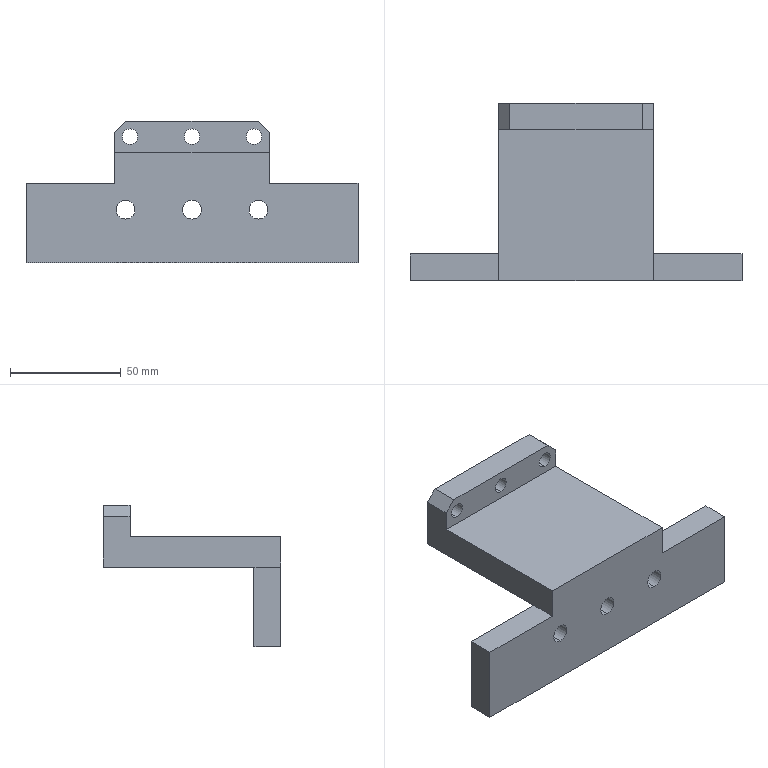Part | NX | 1 solid | 28 faces | box 150 x 80 x 64 mm | volume 151232 mm3 | plane 16 | cylinder 12 | commonest cylinder face diameters 7 x6 8.5 x6
STEP:
#1=CARTESIAN_POINT('',(0.,-28.,-35.75));
#2=VERTEX_POINT('',#1);
#3=CARTESIAN_POINT('',(0.,-28.,-44.25));
#4=VERTEX_POINT('',#3);
#5=CARTESIAN_POINT('',(0.,-28.,-40.));
#6=DIRECTION('',(0.,-1.,0.));
#7=DIRECTION('',(0.,0.,-1.));
#8=AXIS2_PLACEMENT_3D('',#5,#6,#7);
#9=CIRCLE('',#8,4.25);
#10=EDGE_CURVE('',#2,#4,#9,.T.);
#11=ORIENTED_EDGE('',*,*,#10,.F.);
#12=CARTESIAN_POINT('',(0.,-40.,-35.75));
#13=VERTEX_POINT('',#12);
#14=CARTESIAN_POINT('',(0.,-40.,-35.75));
#15=DIRECTION('',(0.,-1.,0.));
#16=VECTOR('',#15,1000.);
#17=LINE('',#14,#16);
#18=EDGE_CURVE('',#2,#13,#17,.T.);
#19=ORIENTED_EDGE('',*,*,#18,.T.);
#20=CARTESIAN_POINT('',(0.,-40.,-44.25));
#21=VERTEX_POINT('',#20);
#22=CARTESIAN_POINT('',(0.,-40.,-40.));
#23=DIRECTION('',(0.,-1.,0.));
#24=DIRECTION('',(0.,0.,-1.));
#25=AXIS2_PLACEMENT_3D('',#22,#23,#24);
#26=CIRCLE('',#25,4.25);
#27=EDGE_CURVE('',#13,#21,#26,.T.);
#28=ORIENTED_EDGE('',*,*,#27,.T.);
#29=CARTESIAN_POINT('',(0.,-40.,-44.25));
#30=DIRECTION('',(0.,-1.,0.));
#31=VECTOR('',#30,1000.);
#32=LINE('',#29,#31);
#33=EDGE_CURVE('',#4,#21,#32,.T.);
#34=ORIENTED_EDGE('',*,*,#33,.F.);
#35=EDGE_LOOP('',(#11,#19,#28,#34));
#36=FACE_BOUND('',#35,.T.);
#37=CARTESIAN_POINT('',(0.,-40.,-40.));
#38=DIRECTION('',(0.,-1.,0.));
#39=DIRECTION('',(0.,0.,1.));
#40=AXIS2_PLACEMENT_3D('',#37,#38,#39);
#41=CYLINDRICAL_SURFACE('',#40,4.25);
#42=ADVANCED_FACE('',(#36),#41,.F.);
#43=CARTESIAN_POINT('',(30.,-28.,-35.75));
#44=VERTEX_POINT('',#43);
#45=CARTESIAN_POINT('',(30.,-28.,-44.25));
#46=VERTEX_POINT('',#45);
#47=CARTESIAN_POINT('',(30.,-28.,-40.));
#48=DIRECTION('',(0.,-1.,0.));
#49=DIRECTION('',(0.,0.,-1.));
#50=AXIS2_PLACEMENT_3D('',#47,#48,#49);
#51=CIRCLE('',#50,4.25);
#52=EDGE_CURVE('',#44,#46,#51,.T.);
#53=ORIENTED_EDGE('',*,*,#52,.F.);
#54=CARTESIAN_POINT('',(30.,-40.,-35.75));
#55=VERTEX_POINT('',#54);
#56=CARTESIAN_POINT('',(30.,-40.,-35.75));
#57=DIRECTION('',(0.,-1.,0.));
#58=VECTOR('',#57,1000.);
#59=LINE('',#56,#58);
#60=EDGE_CURVE('',#44,#55,#59,.T.);
#61=ORIENTED_EDGE('',*,*,#60,.T.);
#62=CARTESIAN_POINT('',(30.,-40.,-44.25));
#63=VERTEX_POINT('',#62);
#64=CARTESIAN_POINT('',(30.,-40.,-40.));
#65=DIRECTION('',(0.,-1.,0.));
#66=DIRECTION('',(0.,0.,-1.));
#67=AXIS2_PLACEMENT_3D('',#64,#65,#66);
#68=CIRCLE('',#67,4.25);
#69=EDGE_CURVE('',#55,#63,#68,.T.);
#70=ORIENTED_EDGE('',*,*,#69,.T.);
#71=CARTESIAN_POINT('',(30.,-40.,-44.25));
#72=DIRECTION('',(0.,-1.,0.));
#73=VECTOR('',#72,1000.);
#74=LINE('',#71,#73);
#75=EDGE_CURVE('',#46,#63,#74,.T.);
#76=ORIENTED_EDGE('',*,*,#75,.F.);
#77=EDGE_LOOP('',(#53,#61,#70,#76));
#78=FACE_BOUND('',#77,.T.);
#79=CARTESIAN_POINT('',(30.,-40.,-40.));
#80=DIRECTION('',(0.,-1.,0.));
#81=DIRECTION('',(0.,0.,1.));
#82=AXIS2_PLACEMENT_3D('',#79,#80,#81);
#83=CYLINDRICAL_SURFACE('',#82,4.25);
#84=ADVANCED_FACE('',(#78),#83,.F.);
#85=CARTESIAN_POINT('',(-28.,28.,-10.5));
#86=VERTEX_POINT('',#85);
#87=CARTESIAN_POINT('',(-28.,28.,-3.5));
#88=VERTEX_POINT('',#87);
#89=CARTESIAN_POINT('',(-28.,28.,-7.));
#90=DIRECTION('',(0.,1.,0.));
#91=DIRECTION('',(0.,0.,1.));
#92=AXIS2_PLACEMENT_3D('',#89,#90,#91);
#93=CIRCLE('',#92,3.5);
#94=EDGE_CURVE('',#86,#88,#93,.T.);
#95=ORIENTED_EDGE('',*,*,#94,.F.);
#96=CARTESIAN_POINT('',(-28.,40.,-10.5));
#97=VERTEX_POINT('',#96);
#98=CARTESIAN_POINT('',(-28.,40.,-10.5));
#99=DIRECTION('',(0.,1.,0.));
#100=VECTOR('',#99,1000.);
#101=LINE('',#98,#100);
#102=EDGE_CURVE('',#86,#97,#101,.T.);
#103=ORIENTED_EDGE('',*,*,#102,.T.);
#104=CARTESIAN_POINT('',(-28.,40.,-3.5));
#105=VERTEX_POINT('',#104);
#106=CARTESIAN_POINT('',(-28.,40.,-7.));
#107=DIRECTION('',(0.,1.,0.));
#108=DIRECTION('',(0.,0.,1.));
#109=AXIS2_PLACEMENT_3D('',#106,#107,#108);
#110=CIRCLE('',#109,3.5);
#111=EDGE_CURVE('',#97,#105,#110,.T.);
#112=ORIENTED_EDGE('',*,*,#111,.T.);
#113=CARTESIAN_POINT('',(-28.,40.,-3.5));
#114=DIRECTION('',(0.,1.,0.));
#115=VECTOR('',#114,1000.);
#116=LINE('',#113,#115);
#117=EDGE_CURVE('',#88,#105,#116,.T.);
#118=ORIENTED_EDGE('',*,*,#117,.F.);
#119=EDGE_LOOP('',(#95,#103,#112,#118));
#120=FACE_BOUND('',#119,.T.);
#121=CARTESIAN_POINT('',(-28.,40.,-7.));
#122=DIRECTION('',(0.,1.,0.));
#123=DIRECTION('',(0.,0.,-1.));
#124=AXIS2_PLACEMENT_3D('',#121,#122,#123);
#125=CYLINDRICAL_SURFACE('',#124,3.5);
#126=ADVANCED_FACE('',(#120),#125,.F.);
#127=CARTESIAN_POINT('',(0.,28.,-10.5));
#128=VERTEX_POINT('',#127);
#129=CARTESIAN_POINT('',(0.,28.,-3.5));
#130=VERTEX_POINT('',#129);
#131=CARTESIAN_POINT('',(0.,28.,-7.));
#132=DIRECTION('',(0.,1.,0.));
#133=DIRECTION('',(0.,0.,1.));
#134=AXIS2_PLACEMENT_3D('',#131,#132,#133);
#135=CIRCLE('',#134,3.5);
#136=EDGE_CURVE('',#128,#130,#135,.T.);
#137=ORIENTED_EDGE('',*,*,#136,.F.);
#138=CARTESIAN_POINT('',(0.,40.,-10.5));
#139=VERTEX_POINT('',#138);
#140=CARTESIAN_POINT('',(0.,40.,-10.5));
#141=DIRECTION('',(0.,1.,0.));
#142=VECTOR('',#141,1000.);
#143=LINE('',#140,#142);
#144=EDGE_CURVE('',#128,#139,#143,.T.);
#145=ORIENTED_EDGE('',*,*,#144,.T.);
#146=CARTESIAN_POINT('',(0.,40.,-3.5));
#147=VERTEX_POINT('',#146);
#148=CARTESIAN_POINT('',(0.,40.,-7.));
#149=DIRECTION('',(0.,1.,0.));
#150=DIRECTION('',(0.,0.,1.));
#151=AXIS2_PLACEMENT_3D('',#148,#149,#150);
#152=CIRCLE('',#151,3.5);
#153=EDGE_CURVE('',#139,#147,#152,.T.);
#154=ORIENTED_EDGE('',*,*,#153,.T.);
#155=CARTESIAN_POINT('',(0.,40.,-3.5));
#156=DIRECTION('',(0.,1.,0.));
#157=VECTOR('',#156,1000.);
#158=LINE('',#155,#157);
#159=EDGE_CURVE('',#130,#147,#158,.T.);
#160=ORIENTED_EDGE('',*,*,#159,.F.);
#161=EDGE_LOOP('',(#137,#145,#154,#160));
#162=FACE_BOUND('',#161,.T.);
#163=CARTESIAN_POINT('',(0.,40.,-7.));
#164=DIRECTION('',(0.,1.,0.));
#165=DIRECTION('',(0.,0.,-1.));
#166=AXIS2_PLACEMENT_3D('',#163,#164,#165);
#167=CYLINDRICAL_SURFACE('',#166,3.5);
#168=ADVANCED_FACE('',(#162),#167,.F.);
#169=CARTESIAN_POINT('',(28.,28.,-10.5));
#170=VERTEX_POINT('',#169);
#171=CARTESIAN_POINT('',(28.,28.,-3.5));
#172=VERTEX_POINT('',#171);
#173=CARTESIAN_POINT('',(28.,28.,-7.));
#174=DIRECTION('',(0.,1.,0.));
#175=DIRECTION('',(0.,0.,1.));
#176=AXIS2_PLACEMENT_3D('',#173,#174,#175);
#177=CIRCLE('',#176,3.5);
#178=EDGE_CURVE('',#170,#172,#177,.T.);
#179=ORIENTED_EDGE('',*,*,#178,.F.);
#180=CARTESIAN_POINT('',(28.,40.,-10.5));
#181=VERTEX_POINT('',#180);
#182=CARTESIAN_POINT('',(28.,40.,-10.5));
#183=DIRECTION('',(0.,1.,0.));
#184=VECTOR('',#183,1000.);
#185=LINE('',#182,#184);
#186=EDGE_CURVE('',#170,#181,#185,.T.);
#187=ORIENTED_EDGE('',*,*,#186,.T.);
#188=CARTESIAN_POINT('',(28.,40.,-3.5));
#189=VERTEX_POINT('',#188);
#190=CARTESIAN_POINT('',(28.,40.,-7.));
#191=DIRECTION('',(0.,1.,0.));
#192=DIRECTION('',(0.,0.,1.));
#193=AXIS2_PLACEMENT_3D('',#190,#191,#192);
#194=CIRCLE('',#193,3.5);
#195=EDGE_CURVE('',#181,#189,#194,.T.);
#196=ORIENTED_EDGE('',*,*,#195,.T.);
#197=CARTESIAN_POINT('',(28.,40.,-3.5));
#198=DIRECTION('',(0.,1.,0.));
#199=VECTOR('',#198,1000.);
#200=LINE('',#197,#199);
#201=EDGE_CURVE('',#172,#189,#200,.T.);
#202=ORIENTED_EDGE('',*,*,#201,.F.);
#203=EDGE_LOOP('',(#179,#187,#196,#202));
#204=FACE_BOUND('',#203,.T.);
#205=CARTESIAN_POINT('',(28.,40.,-7.));
#206=DIRECTION('',(0.,1.,0.));
#207=DIRECTION('',(0.,0.,-1.));
#208=AXIS2_PLACEMENT_3D('',#205,#206,#207);
#209=CYLINDRICAL_SURFACE('',#208,3.5);
#210=ADVANCED_FACE('',(#204),#209,.F.);
#211=CARTESIAN_POINT('',(-30.,-28.,-35.75));
#212=VERTEX_POINT('',#211);
#213=CARTESIAN_POINT('',(-30.,-28.,-44.25));
#214=VERTEX_POINT('',#213);
#215=CARTESIAN_POINT('',(-30.,-28.,-40.));
#216=DIRECTION('',(0.,-1.,0.));
#217=DIRECTION('',(0.,0.,-1.));
#218=AXIS2_PLACEMENT_3D('',#215,#216,#217);
#219=CIRCLE('',#218,4.25);
#220=EDGE_CURVE('',#212,#214,#219,.T.);
#221=ORIENTED_EDGE('',*,*,#220,.F.);
#222=CARTESIAN_POINT('',(-30.,-40.,-35.75));
#223=VERTEX_POINT('',#222);
#224=CARTESIAN_POINT('',(-30.,-40.,-35.75));
#225=DIRECTION('',(0.,-1.,0.));
#226=VECTOR('',#225,1000.);
#227=LINE('',#224,#226);
#228=EDGE_CURVE('',#212,#223,#227,.T.);
#229=ORIENTED_EDGE('',*,*,#228,.T.);
#230=CARTESIAN_POINT('',(-30.,-40.,-44.25));
#231=VERTEX_POINT('',#230);
#232=CARTESIAN_POINT('',(-30.,-40.,-40.));
#233=DIRECTION('',(0.,-1.,0.));
#234=DIRECTION('',(0.,0.,-1.));
#235=AXIS2_PLACEMENT_3D('',#232,#233,#234);
#236=CIRCLE('',#235,4.25);
#237=EDGE_CURVE('',#223,#231,#236,.T.);
#238=ORIENTED_EDGE('',*,*,#237,.T.);
#239=CARTESIAN_POINT('',(-30.,-40.,-44.25));
#240=DIRECTION('',(0.,-1.,0.));
#241=VECTOR('',#240,1000.);
#242=LINE('',#239,#241);
#243=EDGE_CURVE('',#214,#231,#242,.T.);
#244=ORIENTED_EDGE('',*,*,#243,.F.);
#245=EDGE_LOOP('',(#221,#229,#238,#244));
#246=FACE_BOUND('',#245,.T.);
#247=CARTESIAN_POINT('',(-30.,-40.,-40.));
#248=DIRECTION('',(0.,-1.,0.));
#249=DIRECTION('',(0.,0.,1.));
#250=AXIS2_PLACEMENT_3D('',#247,#248,#249);
#251=CYLINDRICAL_SURFACE('',#250,4.25);
#252=ADVANCED_FACE('',(#246),#251,.F.);
#253=ORIENTED_EDGE('',*,*,#228,.F.);
#254=CARTESIAN_POINT('',(-30.,-28.,-40.));
#255=DIRECTION('',(0.,-1.,0.));
#256=DIRECTION('',(0.,0.,-1.));
#257=AXIS2_PLACEMENT_3D('',#254,#255,#256);
#258=CIRCLE('',#257,4.25);
#259=EDGE_CURVE('',#214,#212,#258,.T.);
#260=ORIENTED_EDGE('',*,*,#259,.F.);
#261=ORIENTED_EDGE('',*,*,#243,.T.);
#262=CARTESIAN_POINT('',(-30.,-40.,-40.));
#263=DIRECTION('',(0.,-1.,0.));
#264=DIRECTION('',(0.,0.,-1.));
#265=AXIS2_PLACEMENT_3D('',#262,#263,#264);
#266=CIRCLE('',#265,4.25);
#267=EDGE_CURVE('',#231,#223,#266,.T.);
#268=ORIENTED_EDGE('',*,*,#267,.T.);
#269=EDGE_LOOP('',(#253,#260,#261,#268));
#270=FACE_BOUND('',#269,.T.);
#271=CARTESIAN_POINT('',(-30.,-40.,-40.));
#272=DIRECTION('',(0.,-1.,0.));
#273=DIRECTION('',(0.,0.,1.));
#274=AXIS2_PLACEMENT_3D('',#271,#272,#273);
#275=CYLINDRICAL_SURFACE('',#274,4.25);
#276=ADVANCED_FACE('',(#270),#275,.F.);
#277=CARTESIAN_POINT('',(-75.,-40.,-64.));
#278=VERTEX_POINT('',#277);
#279=CARTESIAN_POINT('',(-75.,-40.,-28.));
#280=VERTEX_POINT('',#279);
#281=CARTESIAN_POINT('',(-75.,-40.,0.));
#282=DIRECTION('',(0.,0.,1.));
#283=VECTOR('',#282,1000.);
#284=LINE('',#281,#283);
#285=EDGE_CURVE('',#278,#280,#284,.T.);
#286=ORIENTED_EDGE('',*,*,#285,.T.);
#287=CARTESIAN_POINT('',(-75.,-28.,-28.));
#288=VERTEX_POINT('',#287);
#289=CARTESIAN_POINT('',(-75.,-40.,-28.));
#290=DIRECTION('',(0.,1.,0.));
#291=VECTOR('',#290,1000.);
#292=LINE('',#289,#291);
#293=EDGE_CURVE('',#280,#288,#292,.T.);
#294=ORIENTED_EDGE('',*,*,#293,.T.);
#295=CARTESIAN_POINT('',(-75.,-28.,-64.));
#296=VERTEX_POINT('',#295);
#297=CARTESIAN_POINT('',(-75.,-28.,-64.));
#298=DIRECTION('',(0.,0.,-1.));
#299=VECTOR('',#298,1000.);
#300=LINE('',#297,#299);
#301=EDGE_CURVE('',#288,#296,#300,.T.);
#302=ORIENTED_EDGE('',*,*,#301,.T.);
#303=CARTESIAN_POINT('',(-75.,40.,-64.));
#304=DIRECTION('',(0.,-1.,0.));
#305=VECTOR('',#304,1000.);
#306=LINE('',#303,#305);
#307=EDGE_CURVE('',#296,#278,#306,.T.);
#308=ORIENTED_EDGE('',*,*,#307,.T.);
#309=EDGE_LOOP('',(#286,#294,#302,#308));
#310=FACE_BOUND('',#309,.T.);
#311=CARTESIAN_POINT('',(-75.,40.,0.));
#312=DIRECTION('',(1.,0.,0.));
#313=DIRECTION('',(0.,0.,1.));
#314=AXIS2_PLACEMENT_3D('',#311,#312,#313);
#315=PLANE('',#314);
#316=ADVANCED_FACE('',(#310),#315,.F.);
#317=CARTESIAN_POINT('',(-30.,28.,0.));
#318=VERTEX_POINT('',#317);
#319=CARTESIAN_POINT('',(30.,28.,0.));
#320=VERTEX_POINT('',#319);
#321=CARTESIAN_POINT('',(-75.,28.,0.));
#322=DIRECTION('',(1.,0.,0.));
#323=VECTOR('',#322,1000.);
#324=LINE('',#321,#323);
#325=EDGE_CURVE('',#318,#320,#324,.T.);
#326=ORIENTED_EDGE('',*,*,#325,.T.);
#327=CARTESIAN_POINT('',(30.,40.,0.));
#328=VERTEX_POINT('',#327);
#329=CARTESIAN_POINT('',(30.,40.,0.));
#330=DIRECTION('',(0.,1.,0.));
#331=VECTOR('',#330,1000.);
#332=LINE('',#329,#331);
#333=EDGE_CURVE('',#320,#328,#332,.T.);
#334=ORIENTED_EDGE('',*,*,#333,.T.);
#335=CARTESIAN_POINT('',(-30.,40.,0.));
#336=VERTEX_POINT('',#335);
#337=CARTESIAN_POINT('',(75.,40.,0.));
#338=DIRECTION('',(1.,0.,0.));
#339=VECTOR('',#338,1000.);
#340=LINE('',#337,#339);
#341=EDGE_CURVE('',#336,#328,#340,.T.);
#342=ORIENTED_EDGE('',*,*,#341,.F.);
#343=CARTESIAN_POINT('',(-30.,40.,0.));
#344=DIRECTION('',(0.,-1.,0.));
#345=VECTOR('',#344,1000.);
#346=LINE('',#343,#345);
#347=EDGE_CURVE('',#336,#318,#346,.T.);
#348=ORIENTED_EDGE('',*,*,#347,.T.);
#349=EDGE_LOOP('',(#326,#334,#342,#348));
#350=FACE_BOUND('',#349,.T.);
#351=CARTESIAN_POINT('',(75.,40.,0.));
#352=DIRECTION('',(0.,0.,-1.));
#353=DIRECTION('',(1.,0.,0.));
#354=AXIS2_PLACEMENT_3D('',#351,#352,#353);
#355=PLANE('',#354);
#356=ADVANCED_FACE('',(#350),#355,.F.);
#357=CARTESIAN_POINT('',(75.,-28.,-28.));
#358=VERTEX_POINT('',#357);
#359=CARTESIAN_POINT('',(75.,-28.,-64.));
#360=VERTEX_POINT('',#359);
#361=CARTESIAN_POINT('',(75.,-28.,-64.));
#362=DIRECTION('',(0.,0.,-1.));
#363=VECTOR('',#362,1000.);
#364=LINE('',#361,#363);
#365=EDGE_CURVE('',#358,#360,#364,.T.);
#366=ORIENTED_EDGE('',*,*,#365,.F.);
#367=CARTESIAN_POINT('',(75.,-40.,-28.));
#368=VERTEX_POINT('',#367);
#369=CARTESIAN_POINT('',(75.,-40.,-28.));
#370=DIRECTION('',(0.,1.,0.));
#371=VECTOR('',#370,1000.);
#372=LINE('',#369,#371);
#373=EDGE_CURVE('',#368,#358,#372,.T.);
#374=ORIENTED_EDGE('',*,*,#373,.F.);
#375=CARTESIAN_POINT('',(75.,-40.,-64.));
#376=VERTEX_POINT('',#375);
#377=CARTESIAN_POINT('',(75.,-40.,0.));
#378=DIRECTION('',(0.,0.,-1.));
#379=VECTOR('',#378,1000.);
#380=LINE('',#377,#379);
#381=EDGE_CURVE('',#368,#376,#380,.T.);
#382=ORIENTED_EDGE('',*,*,#381,.T.);
#383=CARTESIAN_POINT('',(75.,40.,-64.));
#384=DIRECTION('',(0.,-1.,0.));
#385=VECTOR('',#384,1000.);
#386=LINE('',#383,#385);
#387=EDGE_CURVE('',#360,#376,#386,.T.);
#388=ORIENTED_EDGE('',*,*,#387,.F.);
#389=EDGE_LOOP('',(#366,#374,#382,#388));
#390=FACE_BOUND('',#389,.T.);
#391=CARTESIAN_POINT('',(75.,40.,0.));
#392=DIRECTION('',(-1.,0.,0.));
#393=DIRECTION('',(0.,0.,-1.));
#394=AXIS2_PLACEMENT_3D('',#391,#392,#393);
#395=PLANE('',#394);
#396=ADVANCED_FACE('',(#390),#395,.F.);
#397=ORIENTED_EDGE('',*,*,#307,.F.);
#398=CARTESIAN_POINT('',(-75.,-28.,-64.));
#399=DIRECTION('',(1.,0.,0.));
#400=VECTOR('',#399,1000.);
#401=LINE('',#398,#400);
#402=EDGE_CURVE('',#296,#360,#401,.T.);
#403=ORIENTED_EDGE('',*,*,#402,.T.);
#404=ORIENTED_EDGE('',*,*,#387,.T.);
#405=CARTESIAN_POINT('',(75.,-40.,-64.));
#406=DIRECTION('',(-1.,0.,0.));
#407=VECTOR('',#406,1000.);
#408=LINE('',#405,#407);
#409=EDGE_CURVE('',#376,#278,#408,.T.);
#410=ORIENTED_EDGE('',*,*,#409,.T.);
#411=EDGE_LOOP('',(#397,#403,#404,#410));
#412=FACE_BOUND('',#411,.T.);
#413=CARTESIAN_POINT('',(75.,40.,-64.));
#414=DIRECTION('',(0.,0.,1.));
#415=DIRECTION('',(-1.,0.,0.));
#416=AXIS2_PLACEMENT_3D('',#413,#414,#415);
#417=PLANE('',#416);
#418=ADVANCED_FACE('',(#412),#417,.F.);
#419=ORIENTED_EDGE('',*,*,#341,.T.);
#420=CARTESIAN_POINT('',(35.,40.,-5.));
#421=VERTEX_POINT('',#420);
#422=CARTESIAN_POINT('',(31.,40.,-1.));
#423=DIRECTION('',(0.7071,0.,-0.7071));
#424=VECTOR('',#423,1000.);
#425=LINE('',#422,#424);
#426=EDGE_CURVE('',#328,#421,#425,.T.);
#427=ORIENTED_EDGE('',*,*,#426,.T.);
#428=CARTESIAN_POINT('',(35.,40.,-28.));
#429=VERTEX_POINT('',#428);
#430=CARTESIAN_POINT('',(35.,40.,0.));
#431=DIRECTION('',(0.,0.,1.));
#432=VECTOR('',#431,1000.);
#433=LINE('',#430,#432);
#434=EDGE_CURVE('',#429,#421,#433,.T.);
#435=ORIENTED_EDGE('',*,*,#434,.F.);
#436=CARTESIAN_POINT('',(-35.,40.,-28.));
#437=VERTEX_POINT('',#436);
#438=CARTESIAN_POINT('',(-75.,40.,-28.));
#439=DIRECTION('',(1.,0.,0.));
#440=VECTOR('',#439,1000.);
#441=LINE('',#438,#440);
#442=EDGE_CURVE('',#437,#429,#441,.T.);
#443=ORIENTED_EDGE('',*,*,#442,.F.);
#444=CARTESIAN_POINT('',(-35.,40.,-5.));
#445=VERTEX_POINT('',#444);
#446=CARTESIAN_POINT('',(-35.,40.,0.));
#447=DIRECTION('',(0.,0.,-1.));
#448=VECTOR('',#447,1000.);
#449=LINE('',#446,#448);
#450=EDGE_CURVE('',#445,#437,#449,.T.);
#451=ORIENTED_EDGE('',*,*,#450,.F.);
#452=CARTESIAN_POINT('',(-31.,40.,-1.));
#453=DIRECTION('',(0.7071,0.,0.7071));
#454=VECTOR('',#453,1000.);
#455=LINE('',#452,#454);
#456=EDGE_CURVE('',#445,#336,#455,.T.);
#457=ORIENTED_EDGE('',*,*,#456,.T.);
#458=EDGE_LOOP('',(#419,#427,#435,#443,#451,#457));
#459=FACE_BOUND('',#458,.T.);
#460=CARTESIAN_POINT('',(-28.,40.,-7.));
#461=DIRECTION('',(0.,1.,0.));
#462=DIRECTION('',(0.,0.,1.));
#463=AXIS2_PLACEMENT_3D('',#460,#461,#462);
#464=CIRCLE('',#463,3.5);
#465=EDGE_CURVE('',#105,#97,#464,.T.);
#466=ORIENTED_EDGE('',*,*,#465,.F.);
#467=ORIENTED_EDGE('',*,*,#111,.F.);
#468=EDGE_LOOP('',(#466,#467));
#469=FACE_BOUND('',#468,.T.);
#470=CARTESIAN_POINT('',(0.,40.,-7.));
#471=DIRECTION('',(0.,1.,0.));
#472=DIRECTION('',(0.,0.,1.));
#473=AXIS2_PLACEMENT_3D('',#470,#471,#472);
#474=CIRCLE('',#473,3.5);
#475=EDGE_CURVE('',#147,#139,#474,.T.);
#476=ORIENTED_EDGE('',*,*,#475,.F.);
#477=ORIENTED_EDGE('',*,*,#153,.F.);
#478=EDGE_LOOP('',(#476,#477));
#479=FACE_BOUND('',#478,.T.);
#480=CARTESIAN_POINT('',(28.,40.,-7.));
#481=DIRECTION('',(0.,1.,0.));
#482=DIRECTION('',(0.,0.,1.));
#483=AXIS2_PLACEMENT_3D('',#480,#481,#482);
#484=CIRCLE('',#483,3.5);
#485=EDGE_CURVE('',#189,#181,#484,.T.);
#486=ORIENTED_EDGE('',*,*,#485,.F.);
#487=ORIENTED_EDGE('',*,*,#195,.F.);
#488=EDGE_LOOP('',(#486,#487));
#489=FACE_BOUND('',#488,.T.);
#490=CARTESIAN_POINT('',(0.,40.,-32.));
#491=DIRECTION('',(0.,1.,0.));
#492=DIRECTION('',(0.,0.,-1.));
#493=AXIS2_PLACEMENT_3D('',#490,#491,#492);
#494=PLANE('',#493);
#495=ADVANCED_FACE('',(#459,#469,#479,#489),#494,.T.);
#496=CARTESIAN_POINT('',(0.,-40.,-40.));
#497=DIRECTION('',(0.,-1.,0.));
#498=DIRECTION('',(0.,0.,-1.));
#499=AXIS2_PLACEMENT_3D('',#496,#497,#498);
#500=CIRCLE('',#499,4.25);
#501=EDGE_CURVE('',#21,#13,#500,.T.);
#502=ORIENTED_EDGE('',*,*,#501,.F.);
#503=ORIENTED_EDGE('',*,*,#27,.F.);
#504=EDGE_LOOP('',(#502,#503));
#505=FACE_BOUND('',#504,.T.);
#506=CARTESIAN_POINT('',(30.,-40.,-40.));
#507=DIRECTION('',(0.,-1.,0.));
#508=DIRECTION('',(0.,0.,-1.));
#509=AXIS2_PLACEMENT_3D('',#506,#507,#508);
#510=CIRCLE('',#509,4.25);
#511=EDGE_CURVE('',#63,#55,#510,.T.);
#512=ORIENTED_EDGE('',*,*,#511,.F.);
#513=ORIENTED_EDGE('',*,*,#69,.F.);
#514=EDGE_LOOP('',(#512,#513));
#515=FACE_BOUND('',#514,.T.);
#516=CARTESIAN_POINT('',(-35.,-40.,-14.));
#517=VERTEX_POINT('',#516);
#518=CARTESIAN_POINT('',(-35.,-40.,-28.));
#519=VERTEX_POINT('',#518);
#520=CARTESIAN_POINT('',(-35.,-40.,0.));
#521=DIRECTION('',(0.,0.,-1.));
#522=VECTOR('',#521,1000.);
#523=LINE('',#520,#522);
#524=EDGE_CURVE('',#517,#519,#523,.T.);
#525=ORIENTED_EDGE('',*,*,#524,.T.);
#526=CARTESIAN_POINT('',(-75.,-40.,-28.));
#527=DIRECTION('',(-1.,0.,0.));
#528=VECTOR('',#527,1000.);
#529=LINE('',#526,#528);
#530=EDGE_CURVE('',#519,#280,#529,.T.);
#531=ORIENTED_EDGE('',*,*,#530,.T.);
#532=ORIENTED_EDGE('',*,*,#285,.F.);
#533=ORIENTED_EDGE('',*,*,#409,.F.);
#534=ORIENTED_EDGE('',*,*,#381,.F.);
#535=CARTESIAN_POINT('',(35.,-40.,-28.));
#536=VERTEX_POINT('',#535);
#537=CARTESIAN_POINT('',(75.,-40.,-28.));
#538=DIRECTION('',(-1.,0.,0.));
#539=VECTOR('',#538,1000.);
#540=LINE('',#537,#539);
#541=EDGE_CURVE('',#368,#536,#540,.T.);
#542=ORIENTED_EDGE('',*,*,#541,.T.);
#543=CARTESIAN_POINT('',(35.,-40.,-14.));
#544=VERTEX_POINT('',#543);
#545=CARTESIAN_POINT('',(35.,-40.,0.));
#546=DIRECTION('',(0.,0.,1.));
#547=VECTOR('',#546,1000.);
#548=LINE('',#545,#547);
#549=EDGE_CURVE('',#536,#544,#548,.T.);
#550=ORIENTED_EDGE('',*,*,#549,.T.);
#551=CARTESIAN_POINT('',(-75.,-40.,-14.));
#552=DIRECTION('',(1.,0.,0.));
#553=VECTOR('',#552,1000.);
#554=LINE('',#551,#553);
#555=EDGE_CURVE('',#517,#544,#554,.T.);
#556=ORIENTED_EDGE('',*,*,#555,.F.);
#557=EDGE_LOOP('',(#525,#531,#532,#533,#534,#542,#550,#556));
#558=FACE_BOUND('',#557,.T.);
#559=ORIENTED_EDGE('',*,*,#267,.F.);
#560=ORIENTED_EDGE('',*,*,#237,.F.);
#561=EDGE_LOOP('',(#559,#560));
#562=FACE_BOUND('',#561,.T.);
#563=CARTESIAN_POINT('',(0.,-40.,-32.));
#564=DIRECTION('',(0.,1.,0.));
#565=DIRECTION('',(0.,0.,-1.));
#566=AXIS2_PLACEMENT_3D('',#563,#564,#565);
#567=PLANE('',#566);
#568=ADVANCED_FACE('',(#505,#515,#558,#562),#567,.F.);
#569=CARTESIAN_POINT('',(-28.,28.,-7.));
#570=DIRECTION('',(0.,1.,0.));
#571=DIRECTION('',(0.,0.,1.));
#572=AXIS2_PLACEMENT_3D('',#569,#570,#571);
#573=CIRCLE('',#572,3.5);
#574=EDGE_CURVE('',#88,#86,#573,.T.);
#575=ORIENTED_EDGE('',*,*,#574,.T.);
#576=ORIENTED_EDGE('',*,*,#94,.T.);
#577=EDGE_LOOP('',(#575,#576));
#578=FACE_BOUND('',#577,.T.);
#579=CARTESIAN_POINT('',(0.,28.,-7.));
#580=DIRECTION('',(0.,1.,0.));
#581=DIRECTION('',(0.,0.,1.));
#582=AXIS2_PLACEMENT_3D('',#579,#580,#581);
#583=CIRCLE('',#582,3.5);
#584=EDGE_CURVE('',#130,#128,#583,.T.);
#585=ORIENTED_EDGE('',*,*,#584,.T.);
#586=ORIENTED_EDGE('',*,*,#136,.T.);
#587=EDGE_LOOP('',(#585,#586));
#588=FACE_BOUND('',#587,.T.);
#589=CARTESIAN_POINT('',(28.,28.,-7.));
#590=DIRECTION('',(0.,1.,0.));
#591=DIRECTION('',(0.,0.,1.));
#592=AXIS2_PLACEMENT_3D('',#589,#590,#591);
#593=CIRCLE('',#592,3.5);
#594=EDGE_CURVE('',#172,#170,#593,.T.);
#595=ORIENTED_EDGE('',*,*,#594,.T.);
#596=ORIENTED_EDGE('',*,*,#178,.T.);
#597=EDGE_LOOP('',(#595,#596));
#598=FACE_BOUND('',#597,.T.);
#599=CARTESIAN_POINT('',(35.,28.,-14.));
#600=VERTEX_POINT('',#599);
#601=CARTESIAN_POINT('',(35.,28.,-5.));
#602=VERTEX_POINT('',#601);
#603=CARTESIAN_POINT('',(35.,28.,0.));
#604=DIRECTION('',(0.,0.,1.));
#605=VECTOR('',#604,1000.);
#606=LINE('',#603,#605);
#607=EDGE_CURVE('',#600,#602,#606,.T.);
#608=ORIENTED_EDGE('',*,*,#607,.T.);
#609=CARTESIAN_POINT('',(30.,28.,0.));
#610=DIRECTION('',(-0.7071,0.,0.7071));
#611=VECTOR('',#610,1000.);
#612=LINE('',#609,#611);
#613=EDGE_CURVE('',#602,#320,#612,.T.);
#614=ORIENTED_EDGE('',*,*,#613,.T.);
#615=ORIENTED_EDGE('',*,*,#325,.F.);
#616=CARTESIAN_POINT('',(-35.,28.,-5.));
#617=VERTEX_POINT('',#616);
#618=CARTESIAN_POINT('',(-35.,28.,-5.));
#619=DIRECTION('',(-0.7071,0.,-0.7071));
#620=VECTOR('',#619,1000.);
#621=LINE('',#618,#620);
#622=EDGE_CURVE('',#318,#617,#621,.T.);
#623=ORIENTED_EDGE('',*,*,#622,.T.);
#624=CARTESIAN_POINT('',(-35.,28.,-14.));
#625=VERTEX_POINT('',#624);
#626=CARTESIAN_POINT('',(-35.,28.,0.));
#627=DIRECTION('',(0.,0.,-1.));
#628=VECTOR('',#627,1000.);
#629=LINE('',#626,#628);
#630=EDGE_CURVE('',#617,#625,#629,.T.);
#631=ORIENTED_EDGE('',*,*,#630,.T.);
#632=CARTESIAN_POINT('',(-75.,28.,-14.));
#633=DIRECTION('',(1.,0.,0.));
#634=VECTOR('',#633,1000.);
#635=LINE('',#632,#634);
#636=EDGE_CURVE('',#625,#600,#635,.T.);
#637=ORIENTED_EDGE('',*,*,#636,.T.);
#638=EDGE_LOOP('',(#608,#614,#615,#623,#631,#637));
#639=FACE_BOUND('',#638,.T.);
#640=CARTESIAN_POINT('',(-75.,28.,0.));
#641=DIRECTION('',(0.,1.,0.));
#642=DIRECTION('',(0.,0.,-1.));
#643=AXIS2_PLACEMENT_3D('',#640,#641,#642);
#644=PLANE('',#643);
#645=ADVANCED_FACE('',(#578,#588,#598,#639),#644,.F.);
#646=ORIENTED_EDGE('',*,*,#636,.F.);
#647=CARTESIAN_POINT('',(-35.,-40.,-14.));
#648=DIRECTION('',(0.,-1.,0.));
#649=VECTOR('',#648,1000.);
#650=LINE('',#647,#649);
#651=EDGE_CURVE('',#625,#517,#650,.T.);
#652=ORIENTED_EDGE('',*,*,#651,.T.);
#653=ORIENTED_EDGE('',*,*,#555,.T.);
#654=CARTESIAN_POINT('',(35.,-40.,-14.));
#655=DIRECTION('',(0.,1.,0.));
#656=VECTOR('',#655,1000.);
#657=LINE('',#654,#656);
#658=EDGE_CURVE('',#544,#600,#657,.T.);
#659=ORIENTED_EDGE('',*,*,#658,.T.);
#660=EDGE_LOOP('',(#646,#652,#653,#659));
#661=FACE_BOUND('',#660,.T.);
#662=CARTESIAN_POINT('',(-75.,-40.,-14.));
#663=DIRECTION('',(0.,0.,-1.));
#664=DIRECTION('',(1.,0.,0.));
#665=AXIS2_PLACEMENT_3D('',#662,#663,#664);
#666=PLANE('',#665);
#667=ADVANCED_FACE('',(#661),#666,.F.);
#668=CARTESIAN_POINT('',(0.,-28.,-40.));
#669=DIRECTION('',(0.,-1.,0.));
#670=DIRECTION('',(0.,0.,-1.));
#671=AXIS2_PLACEMENT_3D('',#668,#669,#670);
#672=CIRCLE('',#671,4.25);
#673=EDGE_CURVE('',#4,#2,#672,.T.);
#674=ORIENTED_EDGE('',*,*,#673,.T.);
#675=ORIENTED_EDGE('',*,*,#10,.T.);
#676=EDGE_LOOP('',(#674,#675));
#677=FACE_BOUND('',#676,.T.);
#678=CARTESIAN_POINT('',(30.,-28.,-40.));
#679=DIRECTION('',(0.,-1.,0.));
#680=DIRECTION('',(0.,0.,-1.));
#681=AXIS2_PLACEMENT_3D('',#678,#679,#680);
#682=CIRCLE('',#681,4.25);
#683=EDGE_CURVE('',#46,#44,#682,.T.);
#684=ORIENTED_EDGE('',*,*,#683,.T.);
#685=ORIENTED_EDGE('',*,*,#52,.T.);
#686=EDGE_LOOP('',(#684,#685));
#687=FACE_BOUND('',#686,.T.);
#688=ORIENTED_EDGE('',*,*,#365,.T.);
#689=ORIENTED_EDGE('',*,*,#402,.F.);
#690=ORIENTED_EDGE('',*,*,#301,.F.);
#691=CARTESIAN_POINT('',(-35.,-28.,-28.));
#692=VERTEX_POINT('',#691);
#693=CARTESIAN_POINT('',(-75.,-28.,-28.));
#694=DIRECTION('',(1.,0.,0.));
#695=VECTOR('',#694,1000.);
#696=LINE('',#693,#695);
#697=EDGE_CURVE('',#288,#692,#696,.T.);
#698=ORIENTED_EDGE('',*,*,#697,.T.);
#699=CARTESIAN_POINT('',(35.,-28.,-28.));
#700=VERTEX_POINT('',#699);
#701=CARTESIAN_POINT('',(-75.,-28.,-28.));
#702=DIRECTION('',(1.,0.,0.));
#703=VECTOR('',#702,1000.);
#704=LINE('',#701,#703);
#705=EDGE_CURVE('',#692,#700,#704,.T.);
#706=ORIENTED_EDGE('',*,*,#705,.T.);
#707=CARTESIAN_POINT('',(-75.,-28.,-28.));
#708=DIRECTION('',(1.,0.,0.));
#709=VECTOR('',#708,1000.);
#710=LINE('',#707,#709);
#711=EDGE_CURVE('',#700,#358,#710,.T.);
#712=ORIENTED_EDGE('',*,*,#711,.T.);
#713=EDGE_LOOP('',(#688,#689,#690,#698,#706,#712));
#714=FACE_BOUND('',#713,.T.);
#715=ORIENTED_EDGE('',*,*,#259,.T.);
#716=ORIENTED_EDGE('',*,*,#220,.T.);
#717=EDGE_LOOP('',(#715,#716));
#718=FACE_BOUND('',#717,.T.);
#719=CARTESIAN_POINT('',(-75.,-28.,-64.));
#720=DIRECTION('',(0.,-1.,0.));
#721=DIRECTION('',(0.,0.,1.));
#722=AXIS2_PLACEMENT_3D('',#719,#720,#721);
#723=PLANE('',#722);
#724=ADVANCED_FACE('',(#677,#687,#714,#718),#723,.F.);
#725=ORIENTED_EDGE('',*,*,#705,.F.);
#726=CARTESIAN_POINT('',(-35.,40.,-28.));
#727=DIRECTION('',(0.,1.,0.));
#728=VECTOR('',#727,1000.);
#729=LINE('',#726,#728);
#730=EDGE_CURVE('',#692,#437,#729,.T.);
#731=ORIENTED_EDGE('',*,*,#730,.T.);
#732=ORIENTED_EDGE('',*,*,#442,.T.);
#733=CARTESIAN_POINT('',(35.,40.,-28.));
#734=DIRECTION('',(0.,-1.,0.));
#735=VECTOR('',#734,1000.);
#736=LINE('',#733,#735);
#737=EDGE_CURVE('',#429,#700,#736,.T.);
#738=ORIENTED_EDGE('',*,*,#737,.T.);
#739=EDGE_LOOP('',(#725,#731,#732,#738));
#740=FACE_BOUND('',#739,.T.);
#741=CARTESIAN_POINT('',(-75.,40.,-28.));
#742=DIRECTION('',(0.,0.,1.));
#743=DIRECTION('',(0.,1.,0.));
#744=AXIS2_PLACEMENT_3D('',#741,#742,#743);
#745=PLANE('',#744);
#746=ADVANCED_FACE('',(#740),#745,.F.);
#747=ORIENTED_EDGE('',*,*,#186,.F.);
#748=ORIENTED_EDGE('',*,*,#594,.F.);
#749=ORIENTED_EDGE('',*,*,#201,.T.);
#750=ORIENTED_EDGE('',*,*,#485,.T.);
#751=EDGE_LOOP('',(#747,#748,#749,#750));
#752=FACE_BOUND('',#751,.T.);
#753=CARTESIAN_POINT('',(28.,40.,-7.));
#754=DIRECTION('',(0.,1.,0.));
#755=DIRECTION('',(0.,0.,-1.));
#756=AXIS2_PLACEMENT_3D('',#753,#754,#755);
#757=CYLINDRICAL_SURFACE('',#756,3.5);
#758=ADVANCED_FACE('',(#752),#757,.F.);
#759=ORIENTED_EDGE('',*,*,#144,.F.);
#760=ORIENTED_EDGE('',*,*,#584,.F.);
#761=ORIENTED_EDGE('',*,*,#159,.T.);
#762=ORIENTED_EDGE('',*,*,#475,.T.);
#763=EDGE_LOOP('',(#759,#760,#761,#762));
#764=FACE_BOUND('',#763,.T.);
#765=CARTESIAN_POINT('',(0.,40.,-7.));
#766=DIRECTION('',(0.,1.,0.));
#767=DIRECTION('',(0.,0.,-1.));
#768=AXIS2_PLACEMENT_3D('',#765,#766,#767);
#769=CYLINDRICAL_SURFACE('',#768,3.5);
#770=ADVANCED_FACE('',(#764),#769,.F.);
#771=ORIENTED_EDGE('',*,*,#102,.F.);
#772=ORIENTED_EDGE('',*,*,#574,.F.);
#773=ORIENTED_EDGE('',*,*,#117,.T.);
#774=ORIENTED_EDGE('',*,*,#465,.T.);
#775=EDGE_LOOP('',(#771,#772,#773,#774));
#776=FACE_BOUND('',#775,.T.);
#777=CARTESIAN_POINT('',(-28.,40.,-7.));
#778=DIRECTION('',(0.,1.,0.));
#779=DIRECTION('',(0.,0.,-1.));
#780=AXIS2_PLACEMENT_3D('',#777,#778,#779);
#781=CYLINDRICAL_SURFACE('',#780,3.5);
#782=ADVANCED_FACE('',(#776),#781,.F.);
#783=CARTESIAN_POINT('',(35.,-40.,-28.));
#784=DIRECTION('',(0.,1.,0.));
#785=VECTOR('',#784,1000.);
#786=LINE('',#783,#785);
#787=EDGE_CURVE('',#536,#700,#786,.T.);
#788=ORIENTED_EDGE('',*,*,#787,.F.);
#789=ORIENTED_EDGE('',*,*,#541,.F.);
#790=ORIENTED_EDGE('',*,*,#373,.T.);
#791=ORIENTED_EDGE('',*,*,#711,.F.);
#792=EDGE_LOOP('',(#788,#789,#790,#791));
#793=FACE_BOUND('',#792,.T.);
#794=CARTESIAN_POINT('',(75.,-40.,-28.));
#795=DIRECTION('',(0.,0.,-1.));
#796=DIRECTION('',(1.,0.,0.));
#797=AXIS2_PLACEMENT_3D('',#794,#795,#796);
#798=PLANE('',#797);
#799=ADVANCED_FACE('',(#793),#798,.F.);
#800=ORIENTED_EDGE('',*,*,#434,.T.);
#801=CARTESIAN_POINT('',(35.,-40.,-5.));
#802=DIRECTION('',(0.,-1.,0.));
#803=VECTOR('',#802,1000.);
#804=LINE('',#801,#803);
#805=EDGE_CURVE('',#421,#602,#804,.T.);
#806=ORIENTED_EDGE('',*,*,#805,.T.);
#807=ORIENTED_EDGE('',*,*,#607,.F.);
#808=ORIENTED_EDGE('',*,*,#658,.F.);
#809=ORIENTED_EDGE('',*,*,#549,.F.);
#810=ORIENTED_EDGE('',*,*,#787,.T.);
#811=ORIENTED_EDGE('',*,*,#737,.F.);
#812=EDGE_LOOP('',(#800,#806,#807,#808,#809,#810,#811));
#813=FACE_BOUND('',#812,.T.);
#814=CARTESIAN_POINT('',(35.,-40.,0.));
#815=DIRECTION('',(-1.,0.,0.));
#816=DIRECTION('',(0.,0.,-1.));
#817=AXIS2_PLACEMENT_3D('',#814,#815,#816);
#818=PLANE('',#817);
#819=ADVANCED_FACE('',(#813),#818,.F.);
#820=ORIENTED_EDGE('',*,*,#293,.F.);
#821=ORIENTED_EDGE('',*,*,#530,.F.);
#822=CARTESIAN_POINT('',(-35.,-40.,-28.));
#823=DIRECTION('',(0.,1.,0.));
#824=VECTOR('',#823,1000.);
#825=LINE('',#822,#824);
#826=EDGE_CURVE('',#519,#692,#825,.T.);
#827=ORIENTED_EDGE('',*,*,#826,.T.);
#828=ORIENTED_EDGE('',*,*,#697,.F.);
#829=EDGE_LOOP('',(#820,#821,#827,#828));
#830=FACE_BOUND('',#829,.T.);
#831=CARTESIAN_POINT('',(-75.,-40.,-28.));
#832=DIRECTION('',(0.,0.,-1.));
#833=DIRECTION('',(1.,0.,0.));
#834=AXIS2_PLACEMENT_3D('',#831,#832,#833);
#835=PLANE('',#834);
#836=ADVANCED_FACE('',(#830),#835,.F.);
#837=ORIENTED_EDGE('',*,*,#630,.F.);
#838=CARTESIAN_POINT('',(-35.,-40.,-5.));
#839=DIRECTION('',(0.,1.,0.));
#840=VECTOR('',#839,1000.);
#841=LINE('',#838,#840);
#842=EDGE_CURVE('',#617,#445,#841,.T.);
#843=ORIENTED_EDGE('',*,*,#842,.T.);
#844=ORIENTED_EDGE('',*,*,#450,.T.);
#845=ORIENTED_EDGE('',*,*,#730,.F.);
#846=ORIENTED_EDGE('',*,*,#826,.F.);
#847=ORIENTED_EDGE('',*,*,#524,.F.);
#848=ORIENTED_EDGE('',*,*,#651,.F.);
#849=EDGE_LOOP('',(#837,#843,#844,#845,#846,#847,#848));
#850=FACE_BOUND('',#849,.T.);
#851=CARTESIAN_POINT('',(-35.,-40.,0.));
#852=DIRECTION('',(1.,0.,0.));
#853=DIRECTION('',(0.,0.,1.));
#854=AXIS2_PLACEMENT_3D('',#851,#852,#853);
#855=PLANE('',#854);
#856=ADVANCED_FACE('',(#850),#855,.F.);
#857=ORIENTED_EDGE('',*,*,#613,.F.);
#858=ORIENTED_EDGE('',*,*,#805,.F.);
#859=ORIENTED_EDGE('',*,*,#426,.F.);
#860=ORIENTED_EDGE('',*,*,#333,.F.);
#861=EDGE_LOOP('',(#857,#858,#859,#860));
#862=FACE_BOUND('',#861,.T.);
#863=CARTESIAN_POINT('',(30.,40.,0.));
#864=DIRECTION('',(-0.7071,0.,-0.7071));
#865=DIRECTION('',(0.,-1.,0.));
#866=AXIS2_PLACEMENT_3D('',#863,#864,#865);
#867=PLANE('',#866);
#868=ADVANCED_FACE('',(#862),#867,.F.);
#869=ORIENTED_EDGE('',*,*,#622,.F.);
#870=ORIENTED_EDGE('',*,*,#347,.F.);
#871=ORIENTED_EDGE('',*,*,#456,.F.);
#872=ORIENTED_EDGE('',*,*,#842,.F.);
#873=EDGE_LOOP('',(#869,#870,#871,#872));
#874=FACE_BOUND('',#873,.T.);
#875=CARTESIAN_POINT('',(-35.,-40.,-5.));
#876=DIRECTION('',(0.7071,0.,-0.7071));
#877=DIRECTION('',(0.,-1.,0.));
#878=AXIS2_PLACEMENT_3D('',#875,#876,#877);
#879=PLANE('',#878);
#880=ADVANCED_FACE('',(#874),#879,.F.);
#881=ORIENTED_EDGE('',*,*,#60,.F.);
#882=ORIENTED_EDGE('',*,*,#683,.F.);
#883=ORIENTED_EDGE('',*,*,#75,.T.);
#884=ORIENTED_EDGE('',*,*,#511,.T.);
#885=EDGE_LOOP('',(#881,#882,#883,#884));
#886=FACE_BOUND('',#885,.T.);
#887=CARTESIAN_POINT('',(30.,-40.,-40.));
#888=DIRECTION('',(0.,-1.,0.));
#889=DIRECTION('',(0.,0.,1.));
#890=AXIS2_PLACEMENT_3D('',#887,#888,#889);
#891=CYLINDRICAL_SURFACE('',#890,4.25);
#892=ADVANCED_FACE('',(#886),#891,.F.);
#893=ORIENTED_EDGE('',*,*,#18,.F.);
#894=ORIENTED_EDGE('',*,*,#673,.F.);
#895=ORIENTED_EDGE('',*,*,#33,.T.);
#896=ORIENTED_EDGE('',*,*,#501,.T.);
#897=EDGE_LOOP('',(#893,#894,#895,#896));
#898=FACE_BOUND('',#897,.T.);
#899=CARTESIAN_POINT('',(0.,-40.,-40.));
#900=DIRECTION('',(0.,-1.,0.));
#901=DIRECTION('',(0.,0.,1.));
#902=AXIS2_PLACEMENT_3D('',#899,#900,#901);
#903=CYLINDRICAL_SURFACE('',#902,4.25);
#904=ADVANCED_FACE('',(#898),#903,.F.);
#905=CLOSED_SHELL('',(#42,#84,#126,#168,#210,#252,#276,#316,#356,#396,#418,#495,#568,#645,#667,#724,#746,#758,#770,#782,#799,#819,#836,#856,#868,#880,#892,#904));
#906=MANIFOLD_SOLID_BREP('',#905);
#907=(LENGTH_UNIT()NAMED_UNIT(*)SI_UNIT(.MILLI.,.METRE.));
#908=UNCERTAINTY_MEASURE_WITH_UNIT(LENGTH_MEASURE(0.00001),#907,'','');
#909=(NAMED_UNIT(*)PLANE_ANGLE_UNIT()SI_UNIT($,.RADIAN.));
#910=(NAMED_UNIT(*)SI_UNIT($,.STERADIAN.)SOLID_ANGLE_UNIT());
#911=(GEOMETRIC_REPRESENTATION_CONTEXT(3)GLOBAL_UNCERTAINTY_ASSIGNED_CONTEXT((#908))GLOBAL_UNIT_ASSIGNED_CONTEXT((#907,#909,#910))REPRESENTATION_CONTEXT('',''));
#912=ADVANCED_BREP_SHAPE_REPRESENTATION('',(#906),#911);